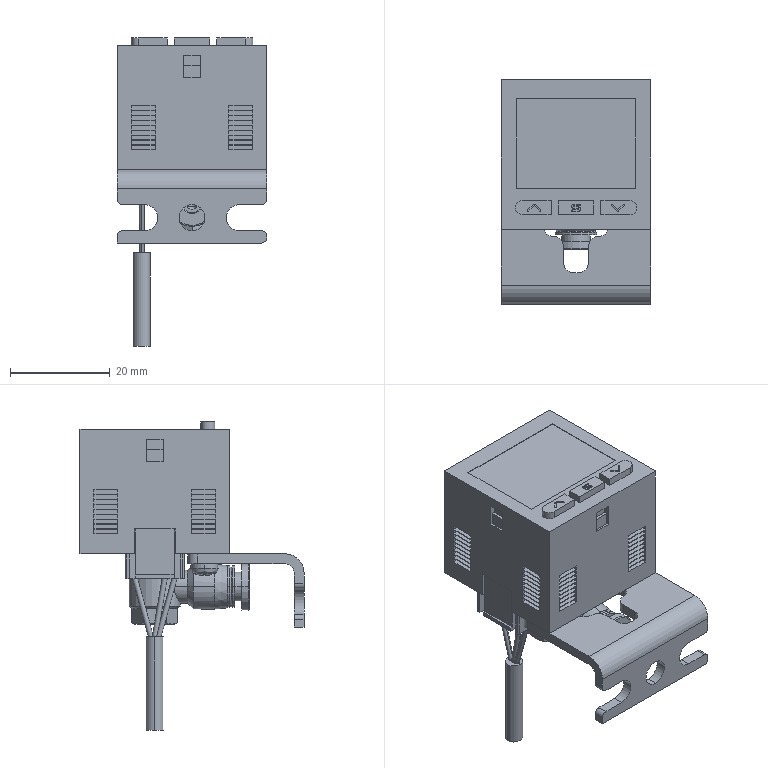Part | SolidWorks | 4 solids | 788 faces | box 30 x 45 x 61.9 mm | volume 25881 mm3 | plane 602 | cylinder 126 | cone 45 | spline 15 | commonest cylinder face diameters 2 x13 0.3 x12 1.6 x8 2.459 x8 4 x8 1 x6